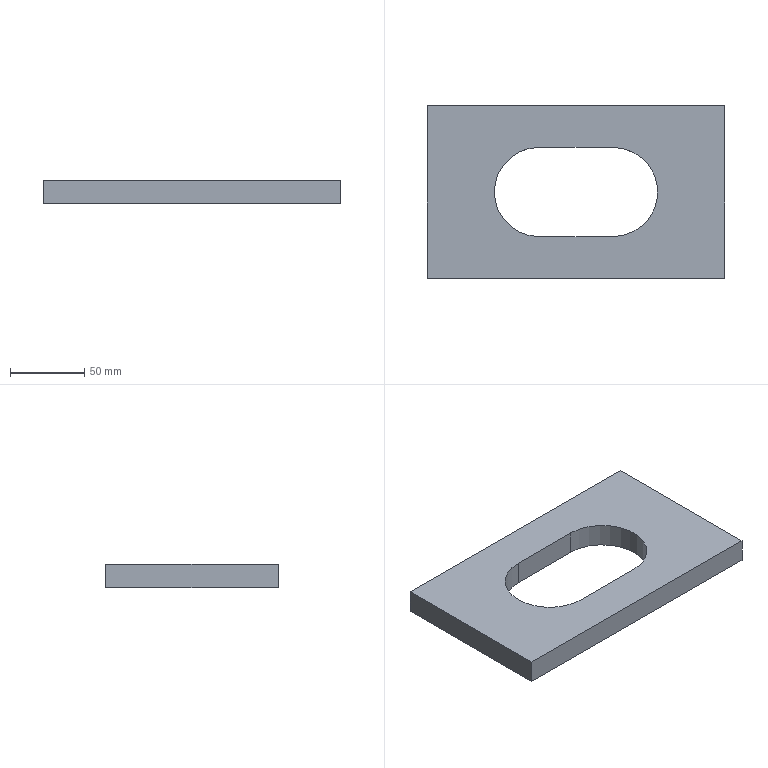Part | SolidWorks | features Extrusion 1 | 1 solid | 11 faces | box 200 x 116 x 16 mm | volume 277961 mm3 | plane 8 | cylinder 3 | commonest cylinder face diameters 60 x3
STEP:
#1=CARTESIAN_POINT('',(0.,30.,16.));
#2=VERTEX_POINT('',#1);
#3=CARTESIAN_POINT('',(-30.,0.,16.));
#4=VERTEX_POINT('',#3);
#5=CARTESIAN_POINT('',(0.,0.,16.));
#6=DIRECTION('',(0.,0.,1.));
#7=DIRECTION('',(1.,0.,0.));
#8=AXIS2_PLACEMENT_3D('',#5,#6,#7);
#9=CIRCLE('',#8,30.);
#10=EDGE_CURVE('',#2,#4,#9,.T.);
#11=ORIENTED_EDGE('',*,*,#10,.T.);
#12=CARTESIAN_POINT('',(-30.,0.,0.));
#13=VERTEX_POINT('',#12);
#14=CARTESIAN_POINT('',(-30.,0.,16.));
#15=DIRECTION('',(0.,0.,-1.));
#16=VECTOR('',#15,1000.);
#17=LINE('',#14,#16);
#18=EDGE_CURVE('',#4,#13,#17,.T.);
#19=ORIENTED_EDGE('',*,*,#18,.T.);
#20=CARTESIAN_POINT('',(0.,30.,0.));
#21=VERTEX_POINT('',#20);
#22=CARTESIAN_POINT('',(0.,0.,0.));
#23=DIRECTION('',(0.,0.,1.));
#24=DIRECTION('',(1.,0.,0.));
#25=AXIS2_PLACEMENT_3D('',#22,#23,#24);
#26=CIRCLE('',#25,30.);
#27=EDGE_CURVE('',#21,#13,#26,.T.);
#28=ORIENTED_EDGE('',*,*,#27,.F.);
#29=CARTESIAN_POINT('',(0.,30.,16.));
#30=DIRECTION('',(0.,0.,-1.));
#31=VECTOR('',#30,1000.);
#32=LINE('',#29,#31);
#33=EDGE_CURVE('',#2,#21,#32,.T.);
#34=ORIENTED_EDGE('',*,*,#33,.F.);
#35=EDGE_LOOP('',(#11,#19,#28,#34));
#36=FACE_OUTER_BOUND('',#35,.T.);
#37=CARTESIAN_POINT('',(0.,0.,16.));
#38=DIRECTION('',(0.,0.,-1.));
#39=DIRECTION('',(-1.,0.,0.));
#40=AXIS2_PLACEMENT_3D('',#37,#38,#39);
#41=CYLINDRICAL_SURFACE('',#40,30.);
#42=ADVANCED_FACE('',(#36),#41,.F.);
#43=CARTESIAN_POINT('',(-75.,58.,16.));
#44=VERTEX_POINT('',#43);
#45=CARTESIAN_POINT('',(-75.,-58.,16.));
#46=VERTEX_POINT('',#45);
#47=CARTESIAN_POINT('',(-75.,58.,16.));
#48=DIRECTION('',(0.,-1.,0.));
#49=VECTOR('',#48,1000.);
#50=LINE('',#47,#49);
#51=EDGE_CURVE('',#44,#46,#50,.T.);
#52=ORIENTED_EDGE('',*,*,#51,.T.);
#53=CARTESIAN_POINT('',(125.,-58.,16.));
#54=VERTEX_POINT('',#53);
#55=CARTESIAN_POINT('',(-75.,-58.,16.));
#56=DIRECTION('',(1.,0.,0.));
#57=VECTOR('',#56,1000.);
#58=LINE('',#55,#57);
#59=EDGE_CURVE('',#46,#54,#58,.T.);
#60=ORIENTED_EDGE('',*,*,#59,.T.);
#61=CARTESIAN_POINT('',(125.,58.,16.));
#62=VERTEX_POINT('',#61);
#63=CARTESIAN_POINT('',(125.,58.,16.));
#64=DIRECTION('',(0.,1.,0.));
#65=VECTOR('',#64,1000.);
#66=LINE('',#63,#65);
#67=EDGE_CURVE('',#54,#62,#66,.T.);
#68=ORIENTED_EDGE('',*,*,#67,.T.);
#69=CARTESIAN_POINT('',(-75.,58.,16.));
#70=DIRECTION('',(-1.,0.,0.));
#71=VECTOR('',#70,1000.);
#72=LINE('',#69,#71);
#73=EDGE_CURVE('',#62,#44,#72,.T.);
#74=ORIENTED_EDGE('',*,*,#73,.T.);
#75=EDGE_LOOP('',(#52,#60,#68,#74));
#76=FACE_OUTER_BOUND('',#75,.T.);
#77=CARTESIAN_POINT('',(0.,-30.,16.));
#78=VERTEX_POINT('',#77);
#79=CARTESIAN_POINT('',(50.,-30.,16.));
#80=VERTEX_POINT('',#79);
#81=CARTESIAN_POINT('',(0.,-30.,16.));
#82=DIRECTION('',(1.,0.,0.));
#83=VECTOR('',#82,1000.);
#84=LINE('',#81,#83);
#85=EDGE_CURVE('',#78,#80,#84,.T.);
#86=ORIENTED_EDGE('',*,*,#85,.F.);
#87=CARTESIAN_POINT('',(0.,0.,16.));
#88=DIRECTION('',(0.,0.,1.));
#89=DIRECTION('',(1.,0.,0.));
#90=AXIS2_PLACEMENT_3D('',#87,#88,#89);
#91=CIRCLE('',#90,30.);
#92=EDGE_CURVE('',#4,#78,#91,.T.);
#93=ORIENTED_EDGE('',*,*,#92,.F.);
#94=ORIENTED_EDGE('',*,*,#10,.F.);
#95=CARTESIAN_POINT('',(50.,30.,16.));
#96=VERTEX_POINT('',#95);
#97=CARTESIAN_POINT('',(0.,30.,16.));
#98=DIRECTION('',(-1.,0.,0.));
#99=VECTOR('',#98,1000.);
#100=LINE('',#97,#99);
#101=EDGE_CURVE('',#96,#2,#100,.T.);
#102=ORIENTED_EDGE('',*,*,#101,.F.);
#103=CARTESIAN_POINT('',(50.,0.,16.));
#104=DIRECTION('',(0.,0.,1.));
#105=DIRECTION('',(1.,0.,0.));
#106=AXIS2_PLACEMENT_3D('',#103,#104,#105);
#107=CIRCLE('',#106,30.);
#108=EDGE_CURVE('',#80,#96,#107,.T.);
#109=ORIENTED_EDGE('',*,*,#108,.F.);
#110=EDGE_LOOP('',(#86,#93,#94,#102,#109));
#111=FACE_BOUND('',#110,.T.);
#112=CARTESIAN_POINT('',(0.,0.,16.));
#113=DIRECTION('',(0.,0.,1.));
#114=DIRECTION('',(1.,0.,0.));
#115=AXIS2_PLACEMENT_3D('',#112,#113,#114);
#116=PLANE('',#115);
#117=ADVANCED_FACE('',(#76,#111),#116,.T.);
#118=CARTESIAN_POINT('',(-75.,58.,0.));
#119=VERTEX_POINT('',#118);
#120=CARTESIAN_POINT('',(-75.,-58.,0.));
#121=VERTEX_POINT('',#120);
#122=CARTESIAN_POINT('',(-75.,58.,0.));
#123=DIRECTION('',(0.,-1.,0.));
#124=VECTOR('',#123,1000.);
#125=LINE('',#122,#124);
#126=EDGE_CURVE('',#119,#121,#125,.T.);
#127=ORIENTED_EDGE('',*,*,#126,.F.);
#128=CARTESIAN_POINT('',(125.,58.,0.));
#129=VERTEX_POINT('',#128);
#130=CARTESIAN_POINT('',(-75.,58.,0.));
#131=DIRECTION('',(-1.,0.,0.));
#132=VECTOR('',#131,1000.);
#133=LINE('',#130,#132);
#134=EDGE_CURVE('',#129,#119,#133,.T.);
#135=ORIENTED_EDGE('',*,*,#134,.F.);
#136=CARTESIAN_POINT('',(125.,-58.,0.));
#137=VERTEX_POINT('',#136);
#138=CARTESIAN_POINT('',(125.,58.,0.));
#139=DIRECTION('',(0.,1.,0.));
#140=VECTOR('',#139,1000.);
#141=LINE('',#138,#140);
#142=EDGE_CURVE('',#137,#129,#141,.T.);
#143=ORIENTED_EDGE('',*,*,#142,.F.);
#144=CARTESIAN_POINT('',(-75.,-58.,0.));
#145=DIRECTION('',(1.,0.,0.));
#146=VECTOR('',#145,1000.);
#147=LINE('',#144,#146);
#148=EDGE_CURVE('',#121,#137,#147,.T.);
#149=ORIENTED_EDGE('',*,*,#148,.F.);
#150=EDGE_LOOP('',(#127,#135,#143,#149));
#151=FACE_OUTER_BOUND('',#150,.T.);
#152=ORIENTED_EDGE('',*,*,#27,.T.);
#153=CARTESIAN_POINT('',(0.,-30.,0.));
#154=VERTEX_POINT('',#153);
#155=CARTESIAN_POINT('',(0.,0.,0.));
#156=DIRECTION('',(0.,0.,1.));
#157=DIRECTION('',(1.,0.,0.));
#158=AXIS2_PLACEMENT_3D('',#155,#156,#157);
#159=CIRCLE('',#158,30.);
#160=EDGE_CURVE('',#13,#154,#159,.T.);
#161=ORIENTED_EDGE('',*,*,#160,.T.);
#162=CARTESIAN_POINT('',(50.,-30.,0.));
#163=VERTEX_POINT('',#162);
#164=CARTESIAN_POINT('',(0.,-30.,0.));
#165=DIRECTION('',(1.,0.,0.));
#166=VECTOR('',#165,1000.);
#167=LINE('',#164,#166);
#168=EDGE_CURVE('',#154,#163,#167,.T.);
#169=ORIENTED_EDGE('',*,*,#168,.T.);
#170=CARTESIAN_POINT('',(50.,30.,0.));
#171=VERTEX_POINT('',#170);
#172=CARTESIAN_POINT('',(50.,0.,0.));
#173=DIRECTION('',(0.,0.,1.));
#174=DIRECTION('',(1.,0.,0.));
#175=AXIS2_PLACEMENT_3D('',#172,#173,#174);
#176=CIRCLE('',#175,30.);
#177=EDGE_CURVE('',#163,#171,#176,.T.);
#178=ORIENTED_EDGE('',*,*,#177,.T.);
#179=CARTESIAN_POINT('',(0.,30.,0.));
#180=DIRECTION('',(-1.,0.,0.));
#181=VECTOR('',#180,1000.);
#182=LINE('',#179,#181);
#183=EDGE_CURVE('',#171,#21,#182,.T.);
#184=ORIENTED_EDGE('',*,*,#183,.T.);
#185=EDGE_LOOP('',(#152,#161,#169,#178,#184));
#186=FACE_BOUND('',#185,.T.);
#187=CARTESIAN_POINT('',(0.,0.,0.));
#188=DIRECTION('',(0.,0.,1.));
#189=DIRECTION('',(1.,0.,0.));
#190=AXIS2_PLACEMENT_3D('',#187,#188,#189);
#191=PLANE('',#190);
#192=ADVANCED_FACE('',(#151,#186),#191,.F.);
#193=ORIENTED_EDGE('',*,*,#126,.T.);
#194=CARTESIAN_POINT('',(-75.,-58.,16.));
#195=DIRECTION('',(0.,0.,-1.));
#196=VECTOR('',#195,1000.);
#197=LINE('',#194,#196);
#198=EDGE_CURVE('',#46,#121,#197,.T.);
#199=ORIENTED_EDGE('',*,*,#198,.F.);
#200=ORIENTED_EDGE('',*,*,#51,.F.);
#201=CARTESIAN_POINT('',(-75.,58.,16.));
#202=DIRECTION('',(0.,0.,-1.));
#203=VECTOR('',#202,1000.);
#204=LINE('',#201,#203);
#205=EDGE_CURVE('',#44,#119,#204,.T.);
#206=ORIENTED_EDGE('',*,*,#205,.T.);
#207=EDGE_LOOP('',(#193,#199,#200,#206));
#208=FACE_OUTER_BOUND('',#207,.T.);
#209=CARTESIAN_POINT('',(-75.,58.,16.));
#210=DIRECTION('',(1.,0.,0.));
#211=DIRECTION('',(0.,1.,0.));
#212=AXIS2_PLACEMENT_3D('',#209,#210,#211);
#213=PLANE('',#212);
#214=ADVANCED_FACE('',(#208),#213,.F.);
#215=ORIENTED_EDGE('',*,*,#148,.T.);
#216=CARTESIAN_POINT('',(125.,-58.,16.));
#217=DIRECTION('',(0.,0.,-1.));
#218=VECTOR('',#217,1000.);
#219=LINE('',#216,#218);
#220=EDGE_CURVE('',#54,#137,#219,.T.);
#221=ORIENTED_EDGE('',*,*,#220,.F.);
#222=ORIENTED_EDGE('',*,*,#59,.F.);
#223=ORIENTED_EDGE('',*,*,#198,.T.);
#224=EDGE_LOOP('',(#215,#221,#222,#223));
#225=FACE_OUTER_BOUND('',#224,.T.);
#226=CARTESIAN_POINT('',(-75.,-58.,16.));
#227=DIRECTION('',(0.,1.,0.));
#228=DIRECTION('',(0.,0.,1.));
#229=AXIS2_PLACEMENT_3D('',#226,#227,#228);
#230=PLANE('',#229);
#231=ADVANCED_FACE('',(#225),#230,.F.);
#232=ORIENTED_EDGE('',*,*,#142,.T.);
#233=CARTESIAN_POINT('',(125.,58.,16.));
#234=DIRECTION('',(0.,0.,-1.));
#235=VECTOR('',#234,1000.);
#236=LINE('',#233,#235);
#237=EDGE_CURVE('',#62,#129,#236,.T.);
#238=ORIENTED_EDGE('',*,*,#237,.F.);
#239=ORIENTED_EDGE('',*,*,#67,.F.);
#240=ORIENTED_EDGE('',*,*,#220,.T.);
#241=EDGE_LOOP('',(#232,#238,#239,#240));
#242=FACE_OUTER_BOUND('',#241,.T.);
#243=CARTESIAN_POINT('',(125.,58.,16.));
#244=DIRECTION('',(-1.,0.,0.));
#245=DIRECTION('',(0.,-1.,0.));
#246=AXIS2_PLACEMENT_3D('',#243,#244,#245);
#247=PLANE('',#246);
#248=ADVANCED_FACE('',(#242),#247,.F.);
#249=ORIENTED_EDGE('',*,*,#134,.T.);
#250=ORIENTED_EDGE('',*,*,#205,.F.);
#251=ORIENTED_EDGE('',*,*,#73,.F.);
#252=ORIENTED_EDGE('',*,*,#237,.T.);
#253=EDGE_LOOP('',(#249,#250,#251,#252));
#254=FACE_OUTER_BOUND('',#253,.T.);
#255=CARTESIAN_POINT('',(-75.,58.,16.));
#256=DIRECTION('',(0.,-1.,0.));
#257=DIRECTION('',(1.,0.,0.));
#258=AXIS2_PLACEMENT_3D('',#255,#256,#257);
#259=PLANE('',#258);
#260=ADVANCED_FACE('',(#254),#259,.F.);
#261=ORIENTED_EDGE('',*,*,#18,.F.);
#262=ORIENTED_EDGE('',*,*,#92,.T.);
#263=CARTESIAN_POINT('',(0.,-30.,16.));
#264=DIRECTION('',(0.,0.,-1.));
#265=VECTOR('',#264,1000.);
#266=LINE('',#263,#265);
#267=EDGE_CURVE('',#78,#154,#266,.T.);
#268=ORIENTED_EDGE('',*,*,#267,.T.);
#269=ORIENTED_EDGE('',*,*,#160,.F.);
#270=EDGE_LOOP('',(#261,#262,#268,#269));
#271=FACE_OUTER_BOUND('',#270,.T.);
#272=CARTESIAN_POINT('',(0.,0.,16.));
#273=DIRECTION('',(0.,0.,-1.));
#274=DIRECTION('',(-1.,0.,0.));
#275=AXIS2_PLACEMENT_3D('',#272,#273,#274);
#276=CYLINDRICAL_SURFACE('',#275,30.);
#277=ADVANCED_FACE('',(#271),#276,.F.);
#278=ORIENTED_EDGE('',*,*,#168,.F.);
#279=ORIENTED_EDGE('',*,*,#267,.F.);
#280=ORIENTED_EDGE('',*,*,#85,.T.);
#281=CARTESIAN_POINT('',(50.,-30.,16.));
#282=DIRECTION('',(0.,0.,-1.));
#283=VECTOR('',#282,1000.);
#284=LINE('',#281,#283);
#285=EDGE_CURVE('',#80,#163,#284,.T.);
#286=ORIENTED_EDGE('',*,*,#285,.T.);
#287=EDGE_LOOP('',(#278,#279,#280,#286));
#288=FACE_OUTER_BOUND('',#287,.T.);
#289=CARTESIAN_POINT('',(0.,-30.,16.));
#290=DIRECTION('',(0.,1.,0.));
#291=DIRECTION('',(-1.,0.,0.));
#292=AXIS2_PLACEMENT_3D('',#289,#290,#291);
#293=PLANE('',#292);
#294=ADVANCED_FACE('',(#288),#293,.T.);
#295=ORIENTED_EDGE('',*,*,#177,.F.);
#296=ORIENTED_EDGE('',*,*,#285,.F.);
#297=ORIENTED_EDGE('',*,*,#108,.T.);
#298=CARTESIAN_POINT('',(50.,30.,16.));
#299=DIRECTION('',(0.,0.,-1.));
#300=VECTOR('',#299,1000.);
#301=LINE('',#298,#300);
#302=EDGE_CURVE('',#96,#171,#301,.T.);
#303=ORIENTED_EDGE('',*,*,#302,.T.);
#304=EDGE_LOOP('',(#295,#296,#297,#303));
#305=FACE_OUTER_BOUND('',#304,.T.);
#306=CARTESIAN_POINT('',(50.,0.,16.));
#307=DIRECTION('',(0.,0.,-1.));
#308=DIRECTION('',(-1.,0.,0.));
#309=AXIS2_PLACEMENT_3D('',#306,#307,#308);
#310=CYLINDRICAL_SURFACE('',#309,30.);
#311=ADVANCED_FACE('',(#305),#310,.F.);
#312=ORIENTED_EDGE('',*,*,#183,.F.);
#313=ORIENTED_EDGE('',*,*,#302,.F.);
#314=ORIENTED_EDGE('',*,*,#101,.T.);
#315=ORIENTED_EDGE('',*,*,#33,.T.);
#316=EDGE_LOOP('',(#312,#313,#314,#315));
#317=FACE_OUTER_BOUND('',#316,.T.);
#318=CARTESIAN_POINT('',(0.,30.,16.));
#319=DIRECTION('',(0.,-1.,0.));
#320=DIRECTION('',(1.,0.,0.));
#321=AXIS2_PLACEMENT_3D('',#318,#319,#320);
#322=PLANE('',#321);
#323=ADVANCED_FACE('',(#317),#322,.T.);
#324=CLOSED_SHELL('',(#42,#117,#192,#214,#231,#248,#260,#277,#294,#311,#323));
#325=MANIFOLD_SOLID_BREP('',#324);
#326=CARTESIAN_POINT('',(0.,0.,0.));
#327=DIRECTION('',(0.,0.,1.));
#328=DIRECTION('',(1.,0.,0.));
#329=AXIS2_PLACEMENT_3D('',#326,#327,#328);
#330=(LENGTH_UNIT()NAMED_UNIT(*)SI_UNIT(.MILLI.,.METRE.));
#331=UNCERTAINTY_MEASURE_WITH_UNIT(LENGTH_MEASURE(0.00001),#330,'','');
#332=(NAMED_UNIT(*)PLANE_ANGLE_UNIT()SI_UNIT($,.RADIAN.));
#333=(NAMED_UNIT(*)SI_UNIT($,.STERADIAN.)SOLID_ANGLE_UNIT());
#334=(GEOMETRIC_REPRESENTATION_CONTEXT(3)GLOBAL_UNCERTAINTY_ASSIGNED_CONTEXT((#331))GLOBAL_UNIT_ASSIGNED_CONTEXT((#330,#332,#333))REPRESENTATION_CONTEXT('',''));
#335=ADVANCED_BREP_SHAPE_REPRESENTATION('',(#325,#329),#334);